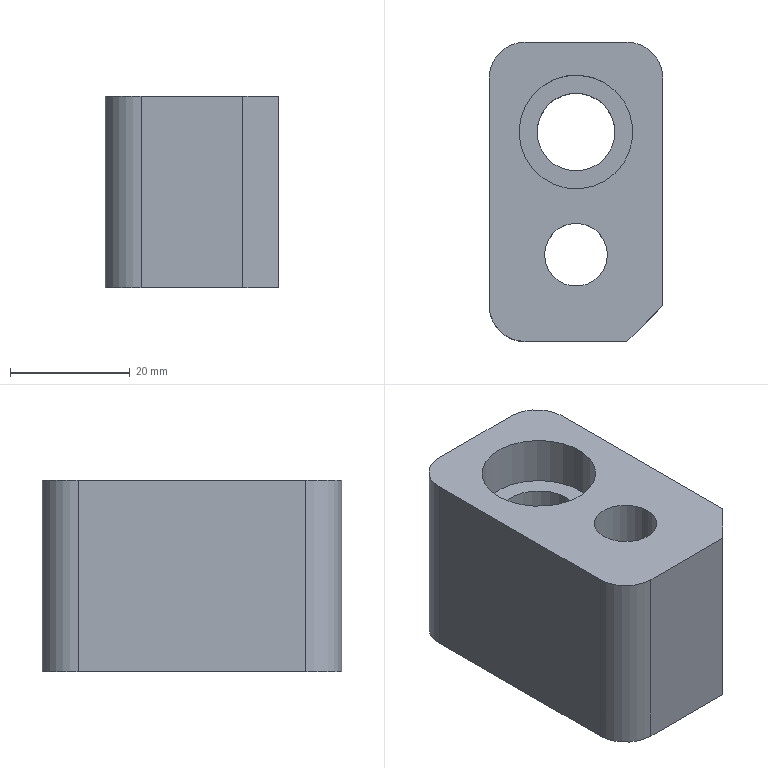Part | STEP file | lll_id102_x_t | 1 solid | 16 faces | box 29 x 50 x 32 mm | volume 34441 mm3 | plane 9 | cylinder 7 | commonest cylinder face diameters 12 x3 10.5 x1 13 x1 17 x1 19 x1
STEP:
#1=CARTESIAN_POINT('',(784.273,-30.,60.5));
#2=VERTEX_POINT('',#1);
#3=CARTESIAN_POINT('',(790.773,-30.,60.5));
#4=DIRECTION('',(0.,0.,1.));
#5=DIRECTION('',(-1.,0.,0.));
#6=AXIS2_PLACEMENT_3D('',#3,#4,#5);
#7=CIRCLE('',#6,6.5);
#8=EDGE_CURVE('',#2,#2,#7,.T.);
#9=ORIENTED_EDGE('',*,*,#8,.T.);
#10=EDGE_LOOP('',(#9));
#11=FACE_BOUND('',#10,.T.);
#12=CARTESIAN_POINT('',(805.273,-21.,60.5));
#13=VERTEX_POINT('',#12);
#14=CARTESIAN_POINT('',(805.273,-59.,60.5));
#15=VERTEX_POINT('',#14);
#16=CARTESIAN_POINT('',(805.273,-30.,60.5));
#17=DIRECTION('',(0.,-1.,0.));
#18=VECTOR('',#17,1.);
#19=LINE('',#16,#18);
#20=EDGE_CURVE('',#13,#15,#19,.T.);
#21=ORIENTED_EDGE('',*,*,#20,.T.);
#22=CARTESIAN_POINT('',(799.273,-65.,60.5));
#23=VERTEX_POINT('',#22);
#24=CARTESIAN_POINT('',(799.273,-65.,60.5));
#25=DIRECTION('',(-0.7071,-0.7071,0.));
#26=VECTOR('',#25,1.);
#27=LINE('',#24,#26);
#28=EDGE_CURVE('',#15,#23,#27,.T.);
#29=ORIENTED_EDGE('',*,*,#28,.T.);
#30=CARTESIAN_POINT('',(782.273,-65.,60.5));
#31=VERTEX_POINT('',#30);
#32=CARTESIAN_POINT('',(790.773,-65.,60.5));
#33=DIRECTION('',(-1.,0.,0.));
#34=VECTOR('',#33,1.);
#35=LINE('',#32,#34);
#36=EDGE_CURVE('',#23,#31,#35,.T.);
#37=ORIENTED_EDGE('',*,*,#36,.T.);
#38=CARTESIAN_POINT('',(776.273,-59.,60.5));
#39=VERTEX_POINT('',#38);
#40=CARTESIAN_POINT('',(782.273,-59.,60.5));
#41=DIRECTION('',(0.,0.,-1.));
#42=DIRECTION('',(-1.,0.,0.));
#43=AXIS2_PLACEMENT_3D('',#40,#41,#42);
#44=CIRCLE('',#43,6.);
#45=EDGE_CURVE('',#31,#39,#44,.T.);
#46=ORIENTED_EDGE('',*,*,#45,.T.);
#47=CARTESIAN_POINT('',(776.273,-21.,60.5));
#48=VERTEX_POINT('',#47);
#49=CARTESIAN_POINT('',(776.273,-30.,60.5));
#50=DIRECTION('',(0.,1.,0.));
#51=VECTOR('',#50,1.);
#52=LINE('',#49,#51);
#53=EDGE_CURVE('',#39,#48,#52,.T.);
#54=ORIENTED_EDGE('',*,*,#53,.T.);
#55=CARTESIAN_POINT('',(782.273,-15.,60.5));
#56=VERTEX_POINT('',#55);
#57=CARTESIAN_POINT('',(782.273,-21.,60.5));
#58=DIRECTION('',(0.,0.,-1.));
#59=DIRECTION('',(-1.,0.,0.));
#60=AXIS2_PLACEMENT_3D('',#57,#58,#59);
#61=CIRCLE('',#60,6.);
#62=EDGE_CURVE('',#48,#56,#61,.T.);
#63=ORIENTED_EDGE('',*,*,#62,.T.);
#64=CARTESIAN_POINT('',(799.273,-15.,60.5));
#65=VERTEX_POINT('',#64);
#66=CARTESIAN_POINT('',(790.773,-15.,60.5));
#67=DIRECTION('',(1.,0.,0.));
#68=VECTOR('',#67,1.);
#69=LINE('',#66,#68);
#70=EDGE_CURVE('',#56,#65,#69,.T.);
#71=ORIENTED_EDGE('',*,*,#70,.T.);
#72=CARTESIAN_POINT('',(799.273,-21.,60.5));
#73=DIRECTION('',(0.,0.,-1.));
#74=DIRECTION('',(-1.,0.,0.));
#75=AXIS2_PLACEMENT_3D('',#72,#73,#74);
#76=CIRCLE('',#75,6.);
#77=EDGE_CURVE('',#65,#13,#76,.T.);
#78=ORIENTED_EDGE('',*,*,#77,.T.);
#79=EDGE_LOOP('',(#21,#29,#37,#46,#54,#63,#71,#78));
#80=FACE_BOUND('',#79,.T.);
#81=CARTESIAN_POINT('',(782.273,-50.5,60.5));
#82=VERTEX_POINT('',#81);
#83=CARTESIAN_POINT('',(790.773,-50.5,60.5));
#84=DIRECTION('',(0.,0.,-1.));
#85=DIRECTION('',(-1.,0.,0.));
#86=AXIS2_PLACEMENT_3D('',#83,#84,#85);
#87=CIRCLE('',#86,8.5);
#88=EDGE_CURVE('',#82,#82,#87,.T.);
#89=ORIENTED_EDGE('',*,*,#88,.F.);
#90=EDGE_LOOP('',(#89));
#91=FACE_BOUND('',#90,.T.);
#92=CARTESIAN_POINT('',(858.913,-61.225,60.5));
#93=DIRECTION('',(0.,0.,1.));
#94=DIRECTION('',(1.,0.,0.));
#95=AXIS2_PLACEMENT_3D('',#92,#93,#94);
#96=PLANE('',#95);
#97=ADVANCED_FACE('',(#11,#80,#91),#96,.F.);
#98=CARTESIAN_POINT('',(781.273,-30.,92.5));
#99=VERTEX_POINT('',#98);
#100=CARTESIAN_POINT('',(790.773,-30.,92.5));
#101=DIRECTION('',(0.,0.,1.));
#102=DIRECTION('',(-1.,0.,0.));
#103=AXIS2_PLACEMENT_3D('',#100,#101,#102);
#104=CIRCLE('',#103,9.5);
#105=EDGE_CURVE('',#99,#99,#104,.T.);
#106=ORIENTED_EDGE('',*,*,#105,.F.);
#107=EDGE_LOOP('',(#106));
#108=FACE_BOUND('',#107,.T.);
#109=CARTESIAN_POINT('',(785.523,-50.5,92.5));
#110=VERTEX_POINT('',#109);
#111=CARTESIAN_POINT('',(790.773,-50.5,92.5));
#112=DIRECTION('',(0.,0.,-1.));
#113=DIRECTION('',(-1.,0.,0.));
#114=AXIS2_PLACEMENT_3D('',#111,#112,#113);
#115=CIRCLE('',#114,5.25);
#116=EDGE_CURVE('',#110,#110,#115,.T.);
#117=ORIENTED_EDGE('',*,*,#116,.T.);
#118=EDGE_LOOP('',(#117));
#119=FACE_BOUND('',#118,.T.);
#120=CARTESIAN_POINT('',(782.273,-65.,92.5));
#121=VERTEX_POINT('',#120);
#122=CARTESIAN_POINT('',(799.273,-65.,92.5));
#123=VERTEX_POINT('',#122);
#124=CARTESIAN_POINT('',(790.773,-65.,92.5));
#125=DIRECTION('',(1.,0.,0.));
#126=VECTOR('',#125,1.);
#127=LINE('',#124,#126);
#128=EDGE_CURVE('',#121,#123,#127,.T.);
#129=ORIENTED_EDGE('',*,*,#128,.T.);
#130=CARTESIAN_POINT('',(805.273,-59.,92.5));
#131=VERTEX_POINT('',#130);
#132=CARTESIAN_POINT('',(830.981,-33.293,92.5));
#133=DIRECTION('',(0.7071,0.7071,0.));
#134=VECTOR('',#133,1.);
#135=LINE('',#132,#134);
#136=EDGE_CURVE('',#123,#131,#135,.T.);
#137=ORIENTED_EDGE('',*,*,#136,.T.);
#138=CARTESIAN_POINT('',(805.273,-21.,92.5));
#139=VERTEX_POINT('',#138);
#140=CARTESIAN_POINT('',(805.273,-30.,92.5));
#141=DIRECTION('',(0.,1.,0.));
#142=VECTOR('',#141,1.);
#143=LINE('',#140,#142);
#144=EDGE_CURVE('',#131,#139,#143,.T.);
#145=ORIENTED_EDGE('',*,*,#144,.T.);
#146=CARTESIAN_POINT('',(799.273,-15.,92.5));
#147=VERTEX_POINT('',#146);
#148=CARTESIAN_POINT('',(799.273,-21.,92.5));
#149=DIRECTION('',(0.,0.,1.));
#150=DIRECTION('',(-1.,0.,0.));
#151=AXIS2_PLACEMENT_3D('',#148,#149,#150);
#152=CIRCLE('',#151,6.);
#153=EDGE_CURVE('',#139,#147,#152,.T.);
#154=ORIENTED_EDGE('',*,*,#153,.T.);
#155=CARTESIAN_POINT('',(782.273,-15.,92.5));
#156=VERTEX_POINT('',#155);
#157=CARTESIAN_POINT('',(790.773,-15.,92.5));
#158=DIRECTION('',(-1.,0.,0.));
#159=VECTOR('',#158,1.);
#160=LINE('',#157,#159);
#161=EDGE_CURVE('',#147,#156,#160,.T.);
#162=ORIENTED_EDGE('',*,*,#161,.T.);
#163=CARTESIAN_POINT('',(776.273,-21.,92.5));
#164=VERTEX_POINT('',#163);
#165=CARTESIAN_POINT('',(782.273,-21.,92.5));
#166=DIRECTION('',(0.,0.,1.));
#167=DIRECTION('',(-1.,0.,0.));
#168=AXIS2_PLACEMENT_3D('',#165,#166,#167);
#169=CIRCLE('',#168,6.);
#170=EDGE_CURVE('',#156,#164,#169,.T.);
#171=ORIENTED_EDGE('',*,*,#170,.T.);
#172=CARTESIAN_POINT('',(776.273,-59.,92.5));
#173=VERTEX_POINT('',#172);
#174=CARTESIAN_POINT('',(776.273,-30.,92.5));
#175=DIRECTION('',(0.,-1.,0.));
#176=VECTOR('',#175,1.);
#177=LINE('',#174,#176);
#178=EDGE_CURVE('',#164,#173,#177,.T.);
#179=ORIENTED_EDGE('',*,*,#178,.T.);
#180=CARTESIAN_POINT('',(782.273,-59.,92.5));
#181=DIRECTION('',(0.,0.,1.));
#182=DIRECTION('',(-1.,0.,0.));
#183=AXIS2_PLACEMENT_3D('',#180,#181,#182);
#184=CIRCLE('',#183,6.);
#185=EDGE_CURVE('',#173,#121,#184,.T.);
#186=ORIENTED_EDGE('',*,*,#185,.T.);
#187=EDGE_LOOP('',(#129,#137,#145,#154,#162,#171,#179,#186));
#188=FACE_BOUND('',#187,.T.);
#189=CARTESIAN_POINT('',(858.913,-61.225,92.5));
#190=DIRECTION('',(0.,0.,1.));
#191=DIRECTION('',(1.,0.,0.));
#192=AXIS2_PLACEMENT_3D('',#189,#190,#191);
#193=PLANE('',#192);
#194=ADVANCED_FACE('',(#108,#119,#188),#193,.T.);
#195=ORIENTED_EDGE('',*,*,#161,.F.);
#196=CARTESIAN_POINT('',(799.273,-15.,-8.5));
#197=DIRECTION('',(0.,0.,-1.));
#198=VECTOR('',#197,1.);
#199=LINE('',#196,#198);
#200=EDGE_CURVE('',#147,#65,#199,.T.);
#201=ORIENTED_EDGE('',*,*,#200,.T.);
#202=ORIENTED_EDGE('',*,*,#70,.F.);
#203=CARTESIAN_POINT('',(782.273,-15.,-8.5));
#204=DIRECTION('',(0.,0.,1.));
#205=VECTOR('',#204,1.);
#206=LINE('',#203,#205);
#207=EDGE_CURVE('',#56,#156,#206,.T.);
#208=ORIENTED_EDGE('',*,*,#207,.T.);
#209=EDGE_LOOP('',(#195,#201,#202,#208));
#210=FACE_OUTER_BOUND('',#209,.T.);
#211=CARTESIAN_POINT('',(790.773,-15.,-8.5));
#212=DIRECTION('',(0.,1.,0.));
#213=DIRECTION('',(0.,0.,-1.));
#214=AXIS2_PLACEMENT_3D('',#211,#212,#213);
#215=PLANE('',#214);
#216=ADVANCED_FACE('',(#210),#215,.T.);
#217=ORIENTED_EDGE('',*,*,#53,.F.);
#218=CARTESIAN_POINT('',(776.273,-59.,-8.5));
#219=DIRECTION('',(0.,0.,1.));
#220=VECTOR('',#219,1.);
#221=LINE('',#218,#220);
#222=EDGE_CURVE('',#39,#173,#221,.T.);
#223=ORIENTED_EDGE('',*,*,#222,.T.);
#224=ORIENTED_EDGE('',*,*,#178,.F.);
#225=CARTESIAN_POINT('',(776.273,-21.,-8.5));
#226=DIRECTION('',(0.,0.,-1.));
#227=VECTOR('',#226,1.);
#228=LINE('',#225,#227);
#229=EDGE_CURVE('',#164,#48,#228,.T.);
#230=ORIENTED_EDGE('',*,*,#229,.T.);
#231=EDGE_LOOP('',(#217,#223,#224,#230));
#232=FACE_OUTER_BOUND('',#231,.T.);
#233=CARTESIAN_POINT('',(776.273,-30.,-8.5));
#234=DIRECTION('',(-1.,0.,0.));
#235=DIRECTION('',(0.,0.,1.));
#236=AXIS2_PLACEMENT_3D('',#233,#234,#235);
#237=PLANE('',#236);
#238=ADVANCED_FACE('',(#232),#237,.T.);
#239=ORIENTED_EDGE('',*,*,#36,.F.);
#240=CARTESIAN_POINT('',(799.273,-65.,-8.5));
#241=DIRECTION('',(0.,0.,1.));
#242=VECTOR('',#241,1.);
#243=LINE('',#240,#242);
#244=EDGE_CURVE('',#23,#123,#243,.T.);
#245=ORIENTED_EDGE('',*,*,#244,.T.);
#246=ORIENTED_EDGE('',*,*,#128,.F.);
#247=CARTESIAN_POINT('',(782.273,-65.,-8.5));
#248=DIRECTION('',(0.,0.,-1.));
#249=VECTOR('',#248,1.);
#250=LINE('',#247,#249);
#251=EDGE_CURVE('',#121,#31,#250,.T.);
#252=ORIENTED_EDGE('',*,*,#251,.T.);
#253=EDGE_LOOP('',(#239,#245,#246,#252));
#254=FACE_OUTER_BOUND('',#253,.T.);
#255=CARTESIAN_POINT('',(790.773,-65.,-8.5));
#256=DIRECTION('',(0.,-1.,0.));
#257=DIRECTION('',(0.,0.,1.));
#258=AXIS2_PLACEMENT_3D('',#255,#256,#257);
#259=PLANE('',#258);
#260=ADVANCED_FACE('',(#254),#259,.T.);
#261=ORIENTED_EDGE('',*,*,#144,.F.);
#262=CARTESIAN_POINT('',(805.273,-59.,-8.5));
#263=DIRECTION('',(0.,0.,-1.));
#264=VECTOR('',#263,1.);
#265=LINE('',#262,#264);
#266=EDGE_CURVE('',#131,#15,#265,.T.);
#267=ORIENTED_EDGE('',*,*,#266,.T.);
#268=ORIENTED_EDGE('',*,*,#20,.F.);
#269=CARTESIAN_POINT('',(805.273,-21.,-8.5));
#270=DIRECTION('',(0.,0.,1.));
#271=VECTOR('',#270,1.);
#272=LINE('',#269,#271);
#273=EDGE_CURVE('',#13,#139,#272,.T.);
#274=ORIENTED_EDGE('',*,*,#273,.T.);
#275=EDGE_LOOP('',(#261,#267,#268,#274));
#276=FACE_OUTER_BOUND('',#275,.T.);
#277=CARTESIAN_POINT('',(805.273,-30.,-8.5));
#278=DIRECTION('',(1.,0.,0.));
#279=DIRECTION('',(0.,0.,-1.));
#280=AXIS2_PLACEMENT_3D('',#277,#278,#279);
#281=PLANE('',#280);
#282=ADVANCED_FACE('',(#276),#281,.T.);
#283=ORIENTED_EDGE('',*,*,#116,.F.);
#284=EDGE_LOOP('',(#283));
#285=FACE_BOUND('',#284,.T.);
#286=CARTESIAN_POINT('',(785.523,-50.5,77.5));
#287=VERTEX_POINT('',#286);
#288=CARTESIAN_POINT('',(790.773,-50.5,77.5));
#289=DIRECTION('',(0.,0.,1.));
#290=DIRECTION('',(-1.,0.,0.));
#291=AXIS2_PLACEMENT_3D('',#288,#289,#290);
#292=CIRCLE('',#291,5.25);
#293=EDGE_CURVE('',#287,#287,#292,.T.);
#294=ORIENTED_EDGE('',*,*,#293,.F.);
#295=EDGE_LOOP('',(#294));
#296=FACE_BOUND('',#295,.T.);
#297=CARTESIAN_POINT('',(790.773,-50.5,160.5));
#298=DIRECTION('',(0.,0.,1.));
#299=DIRECTION('',(1.,0.,0.));
#300=AXIS2_PLACEMENT_3D('',#297,#298,#299);
#301=CYLINDRICAL_SURFACE('',#300,5.25);
#302=ADVANCED_FACE('',(#285,#296),#301,.F.);
#303=ORIENTED_EDGE('',*,*,#293,.T.);
#304=EDGE_LOOP('',(#303));
#305=FACE_BOUND('',#304,.T.);
#306=CARTESIAN_POINT('',(782.273,-50.5,77.5));
#307=VERTEX_POINT('',#306);
#308=CARTESIAN_POINT('',(790.773,-50.5,77.5));
#309=DIRECTION('',(0.,0.,1.));
#310=DIRECTION('',(-1.,0.,0.));
#311=AXIS2_PLACEMENT_3D('',#308,#309,#310);
#312=CIRCLE('',#311,8.5);
#313=EDGE_CURVE('',#307,#307,#312,.T.);
#314=ORIENTED_EDGE('',*,*,#313,.F.);
#315=EDGE_LOOP('',(#314));
#316=FACE_BOUND('',#315,.T.);
#317=CARTESIAN_POINT('',(790.773,-50.5,77.5));
#318=DIRECTION('',(0.,0.,1.));
#319=DIRECTION('',(1.,0.,0.));
#320=AXIS2_PLACEMENT_3D('',#317,#318,#319);
#321=PLANE('',#320);
#322=ADVANCED_FACE('',(#305,#316),#321,.F.);
#323=ORIENTED_EDGE('',*,*,#313,.T.);
#324=EDGE_LOOP('',(#323));
#325=FACE_BOUND('',#324,.T.);
#326=ORIENTED_EDGE('',*,*,#88,.T.);
#327=EDGE_LOOP('',(#326));
#328=FACE_BOUND('',#327,.T.);
#329=CARTESIAN_POINT('',(790.773,-50.5,60.5));
#330=DIRECTION('',(0.,0.,1.));
#331=DIRECTION('',(1.,0.,0.));
#332=AXIS2_PLACEMENT_3D('',#329,#330,#331);
#333=CYLINDRICAL_SURFACE('',#332,8.5);
#334=ADVANCED_FACE('',(#325,#328),#333,.F.);
#335=CARTESIAN_POINT('',(784.273,-30.,84.3));
#336=VERTEX_POINT('',#335);
#337=CARTESIAN_POINT('',(790.773,-30.,84.3));
#338=DIRECTION('',(0.,0.,1.));
#339=DIRECTION('',(-1.,0.,0.));
#340=AXIS2_PLACEMENT_3D('',#337,#338,#339);
#341=CIRCLE('',#340,6.5);
#342=EDGE_CURVE('',#336,#336,#341,.T.);
#343=ORIENTED_EDGE('',*,*,#342,.F.);
#344=EDGE_LOOP('',(#343));
#345=FACE_BOUND('',#344,.T.);
#346=CARTESIAN_POINT('',(781.273,-30.,84.3));
#347=VERTEX_POINT('',#346);
#348=CARTESIAN_POINT('',(790.773,-30.,84.3));
#349=DIRECTION('',(0.,0.,-1.));
#350=DIRECTION('',(-1.,0.,0.));
#351=AXIS2_PLACEMENT_3D('',#348,#349,#350);
#352=CIRCLE('',#351,9.5);
#353=EDGE_CURVE('',#347,#347,#352,.T.);
#354=ORIENTED_EDGE('',*,*,#353,.F.);
#355=EDGE_LOOP('',(#354));
#356=FACE_BOUND('',#355,.T.);
#357=CARTESIAN_POINT('',(790.773,-30.,84.3));
#358=DIRECTION('',(0.,0.,1.));
#359=DIRECTION('',(1.,0.,0.));
#360=AXIS2_PLACEMENT_3D('',#357,#358,#359);
#361=PLANE('',#360);
#362=ADVANCED_FACE('',(#345,#356),#361,.T.);
#363=ORIENTED_EDGE('',*,*,#342,.T.);
#364=EDGE_LOOP('',(#363));
#365=FACE_BOUND('',#364,.T.);
#366=ORIENTED_EDGE('',*,*,#8,.F.);
#367=EDGE_LOOP('',(#366));
#368=FACE_BOUND('',#367,.T.);
#369=CARTESIAN_POINT('',(790.773,-30.,124.8));
#370=DIRECTION('',(0.,0.,-1.));
#371=DIRECTION('',(-1.,0.,0.));
#372=AXIS2_PLACEMENT_3D('',#369,#370,#371);
#373=CYLINDRICAL_SURFACE('',#372,6.5);
#374=ADVANCED_FACE('',(#365,#368),#373,.F.);
#375=ORIENTED_EDGE('',*,*,#353,.T.);
#376=EDGE_LOOP('',(#375));
#377=FACE_BOUND('',#376,.T.);
#378=ORIENTED_EDGE('',*,*,#105,.T.);
#379=EDGE_LOOP('',(#378));
#380=FACE_BOUND('',#379,.T.);
#381=CARTESIAN_POINT('',(790.773,-30.,-7.5));
#382=DIRECTION('',(0.,0.,1.));
#383=DIRECTION('',(1.,0.,0.));
#384=AXIS2_PLACEMENT_3D('',#381,#382,#383);
#385=CYLINDRICAL_SURFACE('',#384,9.5);
#386=ADVANCED_FACE('',(#377,#380),#385,.F.);
#387=ORIENTED_EDGE('',*,*,#185,.F.);
#388=ORIENTED_EDGE('',*,*,#222,.F.);
#389=ORIENTED_EDGE('',*,*,#45,.F.);
#390=ORIENTED_EDGE('',*,*,#251,.F.);
#391=EDGE_LOOP('',(#387,#388,#389,#390));
#392=FACE_OUTER_BOUND('',#391,.T.);
#393=CARTESIAN_POINT('',(782.273,-59.,-8.5));
#394=DIRECTION('',(0.,0.,-1.));
#395=DIRECTION('',(1.,0.,0.));
#396=AXIS2_PLACEMENT_3D('',#393,#394,#395);
#397=CYLINDRICAL_SURFACE('',#396,6.);
#398=ADVANCED_FACE('',(#392),#397,.T.);
#399=ORIENTED_EDGE('',*,*,#153,.F.);
#400=ORIENTED_EDGE('',*,*,#273,.F.);
#401=ORIENTED_EDGE('',*,*,#77,.F.);
#402=ORIENTED_EDGE('',*,*,#200,.F.);
#403=EDGE_LOOP('',(#399,#400,#401,#402));
#404=FACE_OUTER_BOUND('',#403,.T.);
#405=CARTESIAN_POINT('',(799.273,-21.,-8.5));
#406=DIRECTION('',(0.,0.,-1.));
#407=DIRECTION('',(1.,0.,0.));
#408=AXIS2_PLACEMENT_3D('',#405,#406,#407);
#409=CYLINDRICAL_SURFACE('',#408,6.);
#410=ADVANCED_FACE('',(#404),#409,.T.);
#411=ORIENTED_EDGE('',*,*,#170,.F.);
#412=ORIENTED_EDGE('',*,*,#207,.F.);
#413=ORIENTED_EDGE('',*,*,#62,.F.);
#414=ORIENTED_EDGE('',*,*,#229,.F.);
#415=EDGE_LOOP('',(#411,#412,#413,#414));
#416=FACE_OUTER_BOUND('',#415,.T.);
#417=CARTESIAN_POINT('',(782.273,-21.,-8.5));
#418=DIRECTION('',(0.,0.,-1.));
#419=DIRECTION('',(1.,0.,0.));
#420=AXIS2_PLACEMENT_3D('',#417,#418,#419);
#421=CYLINDRICAL_SURFACE('',#420,6.);
#422=ADVANCED_FACE('',(#416),#421,.T.);
#423=ORIENTED_EDGE('',*,*,#28,.F.);
#424=ORIENTED_EDGE('',*,*,#266,.F.);
#425=ORIENTED_EDGE('',*,*,#136,.F.);
#426=ORIENTED_EDGE('',*,*,#244,.F.);
#427=EDGE_LOOP('',(#423,#424,#425,#426));
#428=FACE_OUTER_BOUND('',#427,.T.);
#429=CARTESIAN_POINT('',(799.273,-65.,-8.5));
#430=DIRECTION('',(-0.7071,0.7071,0.));
#431=DIRECTION('',(0.,0.,1.));
#432=AXIS2_PLACEMENT_3D('',#429,#430,#431);
#433=PLANE('',#432);
#434=ADVANCED_FACE('',(#428),#433,.F.);
#435=CLOSED_SHELL('',(#97,#194,#216,#238,#260,#282,#302,#322,#334,#362,#374,#386,#398,#410,#422,#434));
#436=MANIFOLD_SOLID_BREP('',#435);
#437=(LENGTH_UNIT()NAMED_UNIT(*)SI_UNIT(.MILLI.,.METRE.));
#438=UNCERTAINTY_MEASURE_WITH_UNIT(LENGTH_MEASURE(0.00002),#437,'','');
#439=(NAMED_UNIT(*)PLANE_ANGLE_UNIT()SI_UNIT($,.RADIAN.));
#440=PLANE_ANGLE_MEASURE_WITH_UNIT(PLANE_ANGLE_MEASURE(0.01745),#439);
#441=DIMENSIONAL_EXPONENTS(0.,0.,0.,0.,0.,0.,0.);
#442=(CONVERSION_BASED_UNIT('DEGREE',#440)NAMED_UNIT(#441)PLANE_ANGLE_UNIT());
#443=(NAMED_UNIT(*)SI_UNIT($,.STERADIAN.)SOLID_ANGLE_UNIT());
#444=(GEOMETRIC_REPRESENTATION_CONTEXT(3)GLOBAL_UNCERTAINTY_ASSIGNED_CONTEXT((#438))GLOBAL_UNIT_ASSIGNED_CONTEXT((#437,#442,#443))REPRESENTATION_CONTEXT('',''));
#445=ADVANCED_BREP_SHAPE_REPRESENTATION('',(#436),#444);